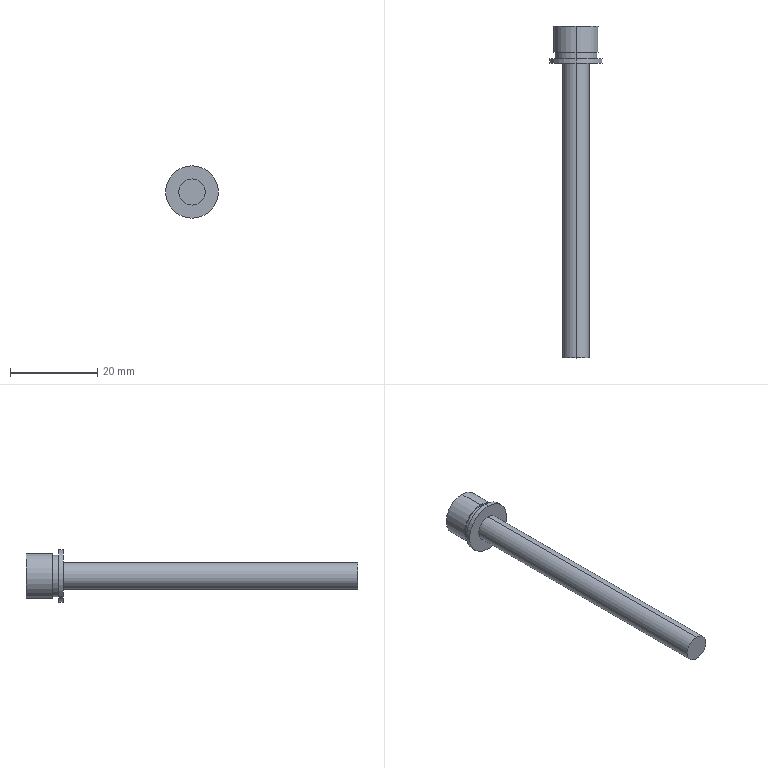Part | SolidWorks | features ICE 3, Revolution 1 | 3 solids | 26 faces | box 12 x 76 x 12 mm | volume 2512 mm3 | plane 14 | cylinder 12 | commonest cylinder face diameters 6 x6 9.6 x2 10.2 x2 12 x2
STEP:
#1=CARTESIAN_POINT('',(0.,-70.,3.));
#2=VERTEX_POINT('',#1);
#3=CARTESIAN_POINT('',(0.,-70.,-3.));
#4=VERTEX_POINT('',#3);
#5=CARTESIAN_POINT('',(0.,-70.,0.));
#6=DIRECTION('',(0.,1.,0.));
#7=DIRECTION('',(0.,0.,1.));
#8=AXIS2_PLACEMENT_3D('',#5,#6,#7);
#9=CIRCLE('',#8,3.);
#10=EDGE_CURVE('',#2,#4,#9,.T.);
#11=ORIENTED_EDGE('',*,*,#10,.T.);
#12=CARTESIAN_POINT('',(0.,0.,-3.));
#13=VERTEX_POINT('',#12);
#14=CARTESIAN_POINT('',(0.,11.322,-3.));
#15=DIRECTION('',(0.,1.,0.));
#16=VECTOR('',#15,1000.);
#17=LINE('',#14,#16);
#18=EDGE_CURVE('',#4,#13,#17,.T.);
#19=ORIENTED_EDGE('',*,*,#18,.T.);
#20=CARTESIAN_POINT('',(0.,0.,3.));
#21=VERTEX_POINT('',#20);
#22=CARTESIAN_POINT('',(0.,0.,0.));
#23=DIRECTION('',(0.,1.,0.));
#24=DIRECTION('',(0.,0.,1.));
#25=AXIS2_PLACEMENT_3D('',#22,#23,#24);
#26=CIRCLE('',#25,3.);
#27=EDGE_CURVE('',#21,#13,#26,.T.);
#28=ORIENTED_EDGE('',*,*,#27,.F.);
#29=CARTESIAN_POINT('',(0.,11.322,3.));
#30=DIRECTION('',(0.,1.,0.));
#31=VECTOR('',#30,1000.);
#32=LINE('',#29,#31);
#33=EDGE_CURVE('',#2,#21,#32,.T.);
#34=ORIENTED_EDGE('',*,*,#33,.F.);
#35=EDGE_LOOP('',(#11,#19,#28,#34));
#36=FACE_OUTER_BOUND('',#35,.T.);
#37=CARTESIAN_POINT('',(0.,11.322,0.));
#38=DIRECTION('',(0.,1.,0.));
#39=DIRECTION('',(0.,0.,1.));
#40=AXIS2_PLACEMENT_3D('',#37,#38,#39);
#41=CYLINDRICAL_SURFACE('',#40,3.);
#42=ADVANCED_FACE('',(#36),#41,.T.);
#43=CARTESIAN_POINT('',(0.,0.,5.1));
#44=VERTEX_POINT('',#43);
#45=CARTESIAN_POINT('',(0.,0.,-5.1));
#46=VERTEX_POINT('',#45);
#47=CARTESIAN_POINT('',(0.,0.,0.));
#48=DIRECTION('',(0.,1.,0.));
#49=DIRECTION('',(0.,0.,1.));
#50=AXIS2_PLACEMENT_3D('',#47,#48,#49);
#51=CIRCLE('',#50,5.1);
#52=EDGE_CURVE('',#44,#46,#51,.T.);
#53=ORIENTED_EDGE('',*,*,#52,.T.);
#54=CARTESIAN_POINT('',(0.,6.,-5.1));
#55=VERTEX_POINT('',#54);
#56=CARTESIAN_POINT('',(0.,11.322,-5.1));
#57=DIRECTION('',(0.,1.,0.));
#58=VECTOR('',#57,1000.);
#59=LINE('',#56,#58);
#60=EDGE_CURVE('',#46,#55,#59,.T.);
#61=ORIENTED_EDGE('',*,*,#60,.T.);
#62=CARTESIAN_POINT('',(0.,6.,5.1));
#63=VERTEX_POINT('',#62);
#64=CARTESIAN_POINT('',(0.,6.,0.));
#65=DIRECTION('',(0.,1.,0.));
#66=DIRECTION('',(0.,0.,1.));
#67=AXIS2_PLACEMENT_3D('',#64,#65,#66);
#68=CIRCLE('',#67,5.1);
#69=EDGE_CURVE('',#63,#55,#68,.T.);
#70=ORIENTED_EDGE('',*,*,#69,.F.);
#71=CARTESIAN_POINT('',(0.,11.322,5.1));
#72=DIRECTION('',(0.,1.,0.));
#73=VECTOR('',#72,1000.);
#74=LINE('',#71,#73);
#75=EDGE_CURVE('',#44,#63,#74,.T.);
#76=ORIENTED_EDGE('',*,*,#75,.F.);
#77=EDGE_LOOP('',(#53,#61,#70,#76));
#78=FACE_OUTER_BOUND('',#77,.T.);
#79=CARTESIAN_POINT('',(0.,11.322,0.));
#80=DIRECTION('',(0.,1.,0.));
#81=DIRECTION('',(0.,0.,1.));
#82=AXIS2_PLACEMENT_3D('',#79,#80,#81);
#83=CYLINDRICAL_SURFACE('',#82,5.1);
#84=ADVANCED_FACE('',(#78),#83,.T.);
#85=CARTESIAN_POINT('',(2.5,6.,-1.443));
#86=VERTEX_POINT('',#85);
#87=CARTESIAN_POINT('',(0.,6.,-2.887));
#88=VERTEX_POINT('',#87);
#89=CARTESIAN_POINT('',(2.5,6.,-1.443));
#90=DIRECTION('',(-0.866,0.,-0.5));
#91=VECTOR('',#90,1000.);
#92=LINE('',#89,#91);
#93=EDGE_CURVE('',#86,#88,#92,.T.);
#94=ORIENTED_EDGE('',*,*,#93,.F.);
#95=CARTESIAN_POINT('',(2.5,6.,1.443));
#96=VERTEX_POINT('',#95);
#97=CARTESIAN_POINT('',(2.5,6.,1.443));
#98=DIRECTION('',(0.,0.,-1.));
#99=VECTOR('',#98,1000.);
#100=LINE('',#97,#99);
#101=EDGE_CURVE('',#96,#86,#100,.T.);
#102=ORIENTED_EDGE('',*,*,#101,.F.);
#103=CARTESIAN_POINT('',(0.,6.,2.887));
#104=VERTEX_POINT('',#103);
#105=CARTESIAN_POINT('',(0.,6.,2.887));
#106=DIRECTION('',(0.866,0.,-0.5));
#107=VECTOR('',#106,1000.);
#108=LINE('',#105,#107);
#109=EDGE_CURVE('',#104,#96,#108,.T.);
#110=ORIENTED_EDGE('',*,*,#109,.F.);
#111=CARTESIAN_POINT('',(-2.5,6.,1.443));
#112=VERTEX_POINT('',#111);
#113=CARTESIAN_POINT('',(-2.5,6.,1.443));
#114=DIRECTION('',(0.866,0.,0.5));
#115=VECTOR('',#114,1000.);
#116=LINE('',#113,#115);
#117=EDGE_CURVE('',#112,#104,#116,.T.);
#118=ORIENTED_EDGE('',*,*,#117,.F.);
#119=CARTESIAN_POINT('',(-2.5,6.,-1.443));
#120=VERTEX_POINT('',#119);
#121=CARTESIAN_POINT('',(-2.5,6.,-1.443));
#122=DIRECTION('',(0.,0.,1.));
#123=VECTOR('',#122,1000.);
#124=LINE('',#121,#123);
#125=EDGE_CURVE('',#120,#112,#124,.T.);
#126=ORIENTED_EDGE('',*,*,#125,.F.);
#127=CARTESIAN_POINT('',(0.,6.,-2.887));
#128=DIRECTION('',(-0.866,0.,0.5));
#129=VECTOR('',#128,1000.);
#130=LINE('',#127,#129);
#131=EDGE_CURVE('',#88,#120,#130,.T.);
#132=ORIENTED_EDGE('',*,*,#131,.F.);
#133=EDGE_LOOP('',(#94,#102,#110,#118,#126,#132));
#134=FACE_BOUND('',#133,.T.);
#135=ORIENTED_EDGE('',*,*,#69,.T.);
#136=CARTESIAN_POINT('',(0.,6.,0.));
#137=DIRECTION('',(0.,1.,0.));
#138=DIRECTION('',(0.,0.,1.));
#139=AXIS2_PLACEMENT_3D('',#136,#137,#138);
#140=CIRCLE('',#139,5.1);
#141=EDGE_CURVE('',#55,#63,#140,.T.);
#142=ORIENTED_EDGE('',*,*,#141,.T.);
#143=EDGE_LOOP('',(#135,#142));
#144=FACE_OUTER_BOUND('',#143,.T.);
#145=CARTESIAN_POINT('',(0.,6.,0.));
#146=DIRECTION('',(0.,1.,0.));
#147=DIRECTION('',(0.,0.,1.));
#148=AXIS2_PLACEMENT_3D('',#145,#146,#147);
#149=PLANE('',#148);
#150=ADVANCED_FACE('',(#134,#144),#149,.T.);
#151=ORIENTED_EDGE('',*,*,#60,.F.);
#152=CARTESIAN_POINT('',(0.,0.,0.));
#153=DIRECTION('',(0.,1.,0.));
#154=DIRECTION('',(0.,0.,1.));
#155=AXIS2_PLACEMENT_3D('',#152,#153,#154);
#156=CIRCLE('',#155,5.1);
#157=EDGE_CURVE('',#46,#44,#156,.T.);
#158=ORIENTED_EDGE('',*,*,#157,.T.);
#159=ORIENTED_EDGE('',*,*,#75,.T.);
#160=ORIENTED_EDGE('',*,*,#141,.F.);
#161=EDGE_LOOP('',(#151,#158,#159,#160));
#162=FACE_OUTER_BOUND('',#161,.T.);
#163=CARTESIAN_POINT('',(0.,11.322,0.));
#164=DIRECTION('',(0.,1.,0.));
#165=DIRECTION('',(0.,0.,1.));
#166=AXIS2_PLACEMENT_3D('',#163,#164,#165);
#167=CYLINDRICAL_SURFACE('',#166,5.1);
#168=ADVANCED_FACE('',(#162),#167,.T.);
#169=ORIENTED_EDGE('',*,*,#27,.T.);
#170=CARTESIAN_POINT('',(0.,0.,0.));
#171=DIRECTION('',(0.,1.,0.));
#172=DIRECTION('',(0.,0.,1.));
#173=AXIS2_PLACEMENT_3D('',#170,#171,#172);
#174=CIRCLE('',#173,3.);
#175=EDGE_CURVE('',#13,#21,#174,.T.);
#176=ORIENTED_EDGE('',*,*,#175,.T.);
#177=EDGE_LOOP('',(#169,#176));
#178=FACE_BOUND('',#177,.T.);
#179=ORIENTED_EDGE('',*,*,#52,.F.);
#180=ORIENTED_EDGE('',*,*,#157,.F.);
#181=EDGE_LOOP('',(#179,#180));
#182=FACE_OUTER_BOUND('',#181,.T.);
#183=CARTESIAN_POINT('',(-5.1,0.,0.));
#184=DIRECTION('',(0.,-1.,0.));
#185=DIRECTION('',(0.,0.,-1.));
#186=AXIS2_PLACEMENT_3D('',#183,#184,#185);
#187=PLANE('',#186);
#188=ADVANCED_FACE('',(#178,#182),#187,.T.);
#189=ORIENTED_EDGE('',*,*,#18,.F.);
#190=CARTESIAN_POINT('',(0.,-70.,0.));
#191=DIRECTION('',(0.,1.,0.));
#192=DIRECTION('',(0.,0.,1.));
#193=AXIS2_PLACEMENT_3D('',#190,#191,#192);
#194=CIRCLE('',#193,3.);
#195=EDGE_CURVE('',#4,#2,#194,.T.);
#196=ORIENTED_EDGE('',*,*,#195,.T.);
#197=ORIENTED_EDGE('',*,*,#33,.T.);
#198=ORIENTED_EDGE('',*,*,#175,.F.);
#199=EDGE_LOOP('',(#189,#196,#197,#198));
#200=FACE_OUTER_BOUND('',#199,.T.);
#201=CARTESIAN_POINT('',(0.,11.322,0.));
#202=DIRECTION('',(0.,1.,0.));
#203=DIRECTION('',(0.,0.,1.));
#204=AXIS2_PLACEMENT_3D('',#201,#202,#203);
#205=CYLINDRICAL_SURFACE('',#204,3.);
#206=ADVANCED_FACE('',(#200),#205,.T.);
#207=ORIENTED_EDGE('',*,*,#10,.F.);
#208=ORIENTED_EDGE('',*,*,#195,.F.);
#209=EDGE_LOOP('',(#207,#208));
#210=FACE_OUTER_BOUND('',#209,.T.);
#211=CARTESIAN_POINT('',(-3.,-70.,0.));
#212=DIRECTION('',(0.,-1.,0.));
#213=DIRECTION('',(0.,0.,-1.));
#214=AXIS2_PLACEMENT_3D('',#211,#212,#213);
#215=PLANE('',#214);
#216=ADVANCED_FACE('',(#210),#215,.T.);
#217=ORIENTED_EDGE('',*,*,#93,.T.);
#218=CARTESIAN_POINT('',(0.,1.,-2.887));
#219=VERTEX_POINT('',#218);
#220=CARTESIAN_POINT('',(0.,1.,-2.887));
#221=DIRECTION('',(0.,1.,0.));
#222=VECTOR('',#221,1000.);
#223=LINE('',#220,#222);
#224=EDGE_CURVE('',#219,#88,#223,.T.);
#225=ORIENTED_EDGE('',*,*,#224,.F.);
#226=CARTESIAN_POINT('',(2.5,1.,-1.443));
#227=VERTEX_POINT('',#226);
#228=CARTESIAN_POINT('',(2.5,1.,-1.443));
#229=DIRECTION('',(-0.866,0.,-0.5));
#230=VECTOR('',#229,1000.);
#231=LINE('',#228,#230);
#232=EDGE_CURVE('',#227,#219,#231,.T.);
#233=ORIENTED_EDGE('',*,*,#232,.F.);
#234=CARTESIAN_POINT('',(2.5,1.,-1.443));
#235=DIRECTION('',(0.,1.,0.));
#236=VECTOR('',#235,1000.);
#237=LINE('',#234,#236);
#238=EDGE_CURVE('',#227,#86,#237,.T.);
#239=ORIENTED_EDGE('',*,*,#238,.T.);
#240=EDGE_LOOP('',(#217,#225,#233,#239));
#241=FACE_OUTER_BOUND('',#240,.T.);
#242=CARTESIAN_POINT('',(2.5,1.,-1.443));
#243=DIRECTION('',(0.5,0.,-0.866));
#244=DIRECTION('',(-0.866,0.,-0.5));
#245=AXIS2_PLACEMENT_3D('',#242,#243,#244);
#246=PLANE('',#245);
#247=ADVANCED_FACE('',(#241),#246,.F.);
#248=ORIENTED_EDGE('',*,*,#101,.T.);
#249=ORIENTED_EDGE('',*,*,#238,.F.);
#250=CARTESIAN_POINT('',(2.5,1.,1.443));
#251=VERTEX_POINT('',#250);
#252=CARTESIAN_POINT('',(2.5,1.,1.443));
#253=DIRECTION('',(0.,0.,-1.));
#254=VECTOR('',#253,1000.);
#255=LINE('',#252,#254);
#256=EDGE_CURVE('',#251,#227,#255,.T.);
#257=ORIENTED_EDGE('',*,*,#256,.F.);
#258=CARTESIAN_POINT('',(2.5,1.,1.443));
#259=DIRECTION('',(0.,1.,0.));
#260=VECTOR('',#259,1000.);
#261=LINE('',#258,#260);
#262=EDGE_CURVE('',#251,#96,#261,.T.);
#263=ORIENTED_EDGE('',*,*,#262,.T.);
#264=EDGE_LOOP('',(#248,#249,#257,#263));
#265=FACE_OUTER_BOUND('',#264,.T.);
#266=CARTESIAN_POINT('',(2.5,1.,1.443));
#267=DIRECTION('',(1.,0.,0.));
#268=DIRECTION('',(0.,0.,-1.));
#269=AXIS2_PLACEMENT_3D('',#266,#267,#268);
#270=PLANE('',#269);
#271=ADVANCED_FACE('',(#265),#270,.F.);
#272=ORIENTED_EDGE('',*,*,#109,.T.);
#273=ORIENTED_EDGE('',*,*,#262,.F.);
#274=CARTESIAN_POINT('',(0.,1.,2.887));
#275=VERTEX_POINT('',#274);
#276=CARTESIAN_POINT('',(0.,1.,2.887));
#277=DIRECTION('',(0.866,0.,-0.5));
#278=VECTOR('',#277,1000.);
#279=LINE('',#276,#278);
#280=EDGE_CURVE('',#275,#251,#279,.T.);
#281=ORIENTED_EDGE('',*,*,#280,.F.);
#282=CARTESIAN_POINT('',(0.,1.,2.887));
#283=DIRECTION('',(0.,1.,0.));
#284=VECTOR('',#283,1000.);
#285=LINE('',#282,#284);
#286=EDGE_CURVE('',#275,#104,#285,.T.);
#287=ORIENTED_EDGE('',*,*,#286,.T.);
#288=EDGE_LOOP('',(#272,#273,#281,#287));
#289=FACE_OUTER_BOUND('',#288,.T.);
#290=CARTESIAN_POINT('',(0.,1.,2.887));
#291=DIRECTION('',(0.5,0.,0.866));
#292=DIRECTION('',(0.866,0.,-0.5));
#293=AXIS2_PLACEMENT_3D('',#290,#291,#292);
#294=PLANE('',#293);
#295=ADVANCED_FACE('',(#289),#294,.F.);
#296=ORIENTED_EDGE('',*,*,#117,.T.);
#297=ORIENTED_EDGE('',*,*,#286,.F.);
#298=CARTESIAN_POINT('',(-2.5,1.,1.443));
#299=VERTEX_POINT('',#298);
#300=CARTESIAN_POINT('',(-2.5,1.,1.443));
#301=DIRECTION('',(0.866,0.,0.5));
#302=VECTOR('',#301,1000.);
#303=LINE('',#300,#302);
#304=EDGE_CURVE('',#299,#275,#303,.T.);
#305=ORIENTED_EDGE('',*,*,#304,.F.);
#306=CARTESIAN_POINT('',(-2.5,1.,1.443));
#307=DIRECTION('',(0.,1.,0.));
#308=VECTOR('',#307,1000.);
#309=LINE('',#306,#308);
#310=EDGE_CURVE('',#299,#112,#309,.T.);
#311=ORIENTED_EDGE('',*,*,#310,.T.);
#312=EDGE_LOOP('',(#296,#297,#305,#311));
#313=FACE_OUTER_BOUND('',#312,.T.);
#314=CARTESIAN_POINT('',(-2.5,1.,1.443));
#315=DIRECTION('',(-0.5,0.,0.866));
#316=DIRECTION('',(0.866,0.,0.5));
#317=AXIS2_PLACEMENT_3D('',#314,#315,#316);
#318=PLANE('',#317);
#319=ADVANCED_FACE('',(#313),#318,.F.);
#320=ORIENTED_EDGE('',*,*,#125,.T.);
#321=ORIENTED_EDGE('',*,*,#310,.F.);
#322=CARTESIAN_POINT('',(-2.5,1.,-1.443));
#323=VERTEX_POINT('',#322);
#324=CARTESIAN_POINT('',(-2.5,1.,-1.443));
#325=DIRECTION('',(0.,0.,1.));
#326=VECTOR('',#325,1000.);
#327=LINE('',#324,#326);
#328=EDGE_CURVE('',#323,#299,#327,.T.);
#329=ORIENTED_EDGE('',*,*,#328,.F.);
#330=CARTESIAN_POINT('',(-2.5,1.,-1.443));
#331=DIRECTION('',(0.,1.,0.));
#332=VECTOR('',#331,1000.);
#333=LINE('',#330,#332);
#334=EDGE_CURVE('',#323,#120,#333,.T.);
#335=ORIENTED_EDGE('',*,*,#334,.T.);
#336=EDGE_LOOP('',(#320,#321,#329,#335));
#337=FACE_OUTER_BOUND('',#336,.T.);
#338=CARTESIAN_POINT('',(-2.5,1.,-1.443));
#339=DIRECTION('',(-1.,0.,0.));
#340=DIRECTION('',(0.,0.,1.));
#341=AXIS2_PLACEMENT_3D('',#338,#339,#340);
#342=PLANE('',#341);
#343=ADVANCED_FACE('',(#337),#342,.F.);
#344=ORIENTED_EDGE('',*,*,#131,.T.);
#345=ORIENTED_EDGE('',*,*,#334,.F.);
#346=CARTESIAN_POINT('',(0.,1.,-2.887));
#347=DIRECTION('',(-0.866,0.,0.5));
#348=VECTOR('',#347,1000.);
#349=LINE('',#346,#348);
#350=EDGE_CURVE('',#219,#323,#349,.T.);
#351=ORIENTED_EDGE('',*,*,#350,.F.);
#352=ORIENTED_EDGE('',*,*,#224,.T.);
#353=EDGE_LOOP('',(#344,#345,#351,#352));
#354=FACE_OUTER_BOUND('',#353,.T.);
#355=CARTESIAN_POINT('',(0.,1.,-2.887));
#356=DIRECTION('',(-0.5,0.,-0.866));
#357=DIRECTION('',(-0.866,0.,0.5));
#358=AXIS2_PLACEMENT_3D('',#355,#356,#357);
#359=PLANE('',#358);
#360=ADVANCED_FACE('',(#354),#359,.F.);
#361=ORIENTED_EDGE('',*,*,#232,.T.);
#362=ORIENTED_EDGE('',*,*,#350,.T.);
#363=ORIENTED_EDGE('',*,*,#328,.T.);
#364=ORIENTED_EDGE('',*,*,#304,.T.);
#365=ORIENTED_EDGE('',*,*,#280,.T.);
#366=ORIENTED_EDGE('',*,*,#256,.T.);
#367=EDGE_LOOP('',(#361,#362,#363,#364,#365,#366));
#368=FACE_OUTER_BOUND('',#367,.T.);
#369=CARTESIAN_POINT('',(0.,1.,0.));
#370=DIRECTION('',(0.,1.,0.));
#371=DIRECTION('',(0.,0.,1.));
#372=AXIS2_PLACEMENT_3D('',#369,#370,#371);
#373=PLANE('',#372);
#374=ADVANCED_FACE('',(#368),#373,.T.);
#375=CLOSED_SHELL('',(#42,#84,#150,#168,#188,#206,#216,#247,#271,#295,#319,#343,#360,#374));
#376=MANIFOLD_SOLID_BREP('',#375);
#377=CARTESIAN_POINT('',(0.,-1.5,3.));
#378=VERTEX_POINT('',#377);
#379=CARTESIAN_POINT('',(0.,-1.5,-3.));
#380=VERTEX_POINT('',#379);
#381=CARTESIAN_POINT('',(0.,-1.5,0.));
#382=DIRECTION('',(0.,-1.,0.));
#383=DIRECTION('',(0.,0.,-1.));
#384=AXIS2_PLACEMENT_3D('',#381,#382,#383);
#385=CIRCLE('',#384,3.);
#386=EDGE_CURVE('',#378,#380,#385,.T.);
#387=ORIENTED_EDGE('',*,*,#386,.T.);
#388=CARTESIAN_POINT('',(0.,0.,-3.));
#389=VERTEX_POINT('',#388);
#390=CARTESIAN_POINT('',(0.,-1.5,-3.));
#391=DIRECTION('',(0.,1.,0.));
#392=VECTOR('',#391,1000.);
#393=LINE('',#390,#392);
#394=EDGE_CURVE('',#380,#389,#393,.T.);
#395=ORIENTED_EDGE('',*,*,#394,.T.);
#396=CARTESIAN_POINT('',(0.,0.,3.));
#397=VERTEX_POINT('',#396);
#398=CARTESIAN_POINT('',(0.,0.,0.));
#399=DIRECTION('',(0.,-1.,0.));
#400=DIRECTION('',(0.,0.,-1.));
#401=AXIS2_PLACEMENT_3D('',#398,#399,#400);
#402=CIRCLE('',#401,3.);
#403=EDGE_CURVE('',#397,#389,#402,.T.);
#404=ORIENTED_EDGE('',*,*,#403,.F.);
#405=CARTESIAN_POINT('',(0.,-1.5,3.));
#406=DIRECTION('',(0.,1.,0.));
#407=VECTOR('',#406,1000.);
#408=LINE('',#405,#407);
#409=EDGE_CURVE('',#378,#397,#408,.T.);
#410=ORIENTED_EDGE('',*,*,#409,.F.);
#411=EDGE_LOOP('',(#387,#395,#404,#410));
#412=FACE_OUTER_BOUND('',#411,.T.);
#413=CARTESIAN_POINT('',(0.,-1.5,0.));
#414=DIRECTION('',(0.,1.,0.));
#415=DIRECTION('',(0.,0.,1.));
#416=AXIS2_PLACEMENT_3D('',#413,#414,#415);
#417=CYLINDRICAL_SURFACE('',#416,3.);
#418=ADVANCED_FACE('',(#412),#417,.F.);
#419=CARTESIAN_POINT('',(0.,-1.5,-4.8));
#420=VERTEX_POINT('',#419);
#421=CARTESIAN_POINT('',(0.,-1.5,4.8));
#422=VERTEX_POINT('',#421);
#423=CARTESIAN_POINT('',(0.,-1.5,0.));
#424=DIRECTION('',(0.,-1.,0.));
#425=DIRECTION('',(0.,0.,-1.));
#426=AXIS2_PLACEMENT_3D('',#423,#424,#425);
#427=CIRCLE('',#426,4.8);
#428=EDGE_CURVE('',#420,#422,#427,.T.);
#429=ORIENTED_EDGE('',*,*,#428,.F.);
#430=CARTESIAN_POINT('',(0.,0.,-4.8));
#431=VERTEX_POINT('',#430);
#432=CARTESIAN_POINT('',(0.,-1.5,-4.8));
#433=DIRECTION('',(0.,1.,0.));
#434=VECTOR('',#433,1000.);
#435=LINE('',#432,#434);
#436=EDGE_CURVE('',#420,#431,#435,.T.);
#437=ORIENTED_EDGE('',*,*,#436,.T.);
#438=CARTESIAN_POINT('',(0.,0.,4.8));
#439=VERTEX_POINT('',#438);
#440=CARTESIAN_POINT('',(0.,0.,0.));
#441=DIRECTION('',(0.,-1.,0.));
#442=DIRECTION('',(0.,0.,-1.));
#443=AXIS2_PLACEMENT_3D('',#440,#441,#442);
#444=CIRCLE('',#443,4.8);
#445=EDGE_CURVE('',#431,#439,#444,.T.);
#446=ORIENTED_EDGE('',*,*,#445,.T.);
#447=CARTESIAN_POINT('',(0.,-1.5,4.8));
#448=DIRECTION('',(0.,1.,0.));
#449=VECTOR('',#448,1000.);
#450=LINE('',#447,#449);
#451=EDGE_CURVE('',#422,#439,#450,.T.);
#452=ORIENTED_EDGE('',*,*,#451,.F.);
#453=EDGE_LOOP('',(#429,#437,#446,#452));
#454=FACE_OUTER_BOUND('',#453,.T.);
#455=CARTESIAN_POINT('',(0.,-1.5,0.));
#456=DIRECTION('',(0.,1.,0.));
#457=DIRECTION('',(0.,0.,1.));
#458=AXIS2_PLACEMENT_3D('',#455,#456,#457);
#459=CYLINDRICAL_SURFACE('',#458,4.8);
#460=ADVANCED_FACE('',(#454),#459,.T.);
#461=CARTESIAN_POINT('',(0.,-1.5,0.));
#462=DIRECTION('',(0.,-1.,0.));
#463=DIRECTION('',(0.,0.,-1.));
#464=AXIS2_PLACEMENT_3D('',#461,#462,#463);
#465=CIRCLE('',#464,4.8);
#466=EDGE_CURVE('',#422,#420,#465,.T.);
#467=ORIENTED_EDGE('',*,*,#466,.T.);
#468=ORIENTED_EDGE('',*,*,#428,.T.);
#469=EDGE_LOOP('',(#467,#468));
#470=FACE_OUTER_BOUND('',#469,.T.);
#471=ORIENTED_EDGE('',*,*,#386,.F.);
#472=CARTESIAN_POINT('',(0.,-1.5,0.));
#473=DIRECTION('',(0.,-1.,0.));
#474=DIRECTION('',(0.,0.,-1.));
#475=AXIS2_PLACEMENT_3D('',#472,#473,#474);
#476=CIRCLE('',#475,3.);
#477=EDGE_CURVE('',#380,#378,#476,.T.);
#478=ORIENTED_EDGE('',*,*,#477,.F.);
#479=EDGE_LOOP('',(#471,#478));
#480=FACE_BOUND('',#479,.T.);
#481=CARTESIAN_POINT('',(0.,-1.5,0.));
#482=DIRECTION('',(0.,-1.,0.));
#483=DIRECTION('',(0.,0.,-1.));
#484=AXIS2_PLACEMENT_3D('',#481,#482,#483);
#485=PLANE('',#484);
#486=ADVANCED_FACE('',(#470,#480),#485,.T.);
#487=CARTESIAN_POINT('',(0.,0.,0.));
#488=DIRECTION('',(0.,-1.,0.));
#489=DIRECTION('',(0.,0.,-1.));
#490=AXIS2_PLACEMENT_3D('',#487,#488,#489);
#491=CIRCLE('',#490,4.8);
#492=EDGE_CURVE('',#439,#431,#491,.T.);
#493=ORIENTED_EDGE('',*,*,#492,.F.);
#494=ORIENTED_EDGE('',*,*,#445,.F.);
#495=EDGE_LOOP('',(#493,#494));
#496=FACE_OUTER_BOUND('',#495,.T.);
#497=ORIENTED_EDGE('',*,*,#403,.T.);
#498=CARTESIAN_POINT('',(0.,0.,0.));
#499=DIRECTION('',(0.,-1.,0.));
#500=DIRECTION('',(0.,0.,-1.));
#501=AXIS2_PLACEMENT_3D('',#498,#499,#500);
#502=CIRCLE('',#501,3.);
#503=EDGE_CURVE('',#389,#397,#502,.T.);
#504=ORIENTED_EDGE('',*,*,#503,.T.);
#505=EDGE_LOOP('',(#497,#504));
#506=FACE_BOUND('',#505,.T.);
#507=CARTESIAN_POINT('',(0.,0.,0.));
#508=DIRECTION('',(0.,-1.,0.));
#509=DIRECTION('',(0.,0.,-1.));
#510=AXIS2_PLACEMENT_3D('',#507,#508,#509);
#511=PLANE('',#510);
#512=ADVANCED_FACE('',(#496,#506),#511,.F.);
#513=ORIENTED_EDGE('',*,*,#436,.F.);
#514=ORIENTED_EDGE('',*,*,#466,.F.);
#515=ORIENTED_EDGE('',*,*,#451,.T.);
#516=ORIENTED_EDGE('',*,*,#492,.T.);
#517=EDGE_LOOP('',(#513,#514,#515,#516));
#518=FACE_OUTER_BOUND('',#517,.T.);
#519=CARTESIAN_POINT('',(0.,-1.5,0.));
#520=DIRECTION('',(0.,1.,0.));
#521=DIRECTION('',(0.,0.,1.));
#522=AXIS2_PLACEMENT_3D('',#519,#520,#521);
#523=CYLINDRICAL_SURFACE('',#522,4.8);
#524=ADVANCED_FACE('',(#518),#523,.T.);
#525=ORIENTED_EDGE('',*,*,#394,.F.);
#526=ORIENTED_EDGE('',*,*,#477,.T.);
#527=ORIENTED_EDGE('',*,*,#409,.T.);
#528=ORIENTED_EDGE('',*,*,#503,.F.);
#529=EDGE_LOOP('',(#525,#526,#527,#528));
#530=FACE_OUTER_BOUND('',#529,.T.);
#531=CARTESIAN_POINT('',(0.,-1.5,0.));
#532=DIRECTION('',(0.,1.,0.));
#533=DIRECTION('',(0.,0.,1.));
#534=AXIS2_PLACEMENT_3D('',#531,#532,#533);
#535=CYLINDRICAL_SURFACE('',#534,3.);
#536=ADVANCED_FACE('',(#530),#535,.F.);
#537=CLOSED_SHELL('',(#418,#460,#486,#512,#524,#536));
#538=MANIFOLD_SOLID_BREP('',#537);
#539=CARTESIAN_POINT('',(0.,-2.5,3.));
#540=VERTEX_POINT('',#539);
#541=CARTESIAN_POINT('',(0.,-2.5,-3.));
#542=VERTEX_POINT('',#541);
#543=CARTESIAN_POINT('',(0.,-2.5,0.));
#544=DIRECTION('',(0.,-1.,0.));
#545=DIRECTION('',(0.,0.,-1.));
#546=AXIS2_PLACEMENT_3D('',#543,#544,#545);
#547=CIRCLE('',#546,3.);
#548=EDGE_CURVE('',#540,#542,#547,.T.);
#549=ORIENTED_EDGE('',*,*,#548,.T.);
#550=CARTESIAN_POINT('',(0.,-1.5,-3.));
#551=VERTEX_POINT('',#550);
#552=CARTESIAN_POINT('',(0.,-2.5,-3.));
#553=DIRECTION('',(0.,1.,0.));
#554=VECTOR('',#553,1000.);
#555=LINE('',#552,#554);
#556=EDGE_CURVE('',#542,#551,#555,.T.);
#557=ORIENTED_EDGE('',*,*,#556,.T.);
#558=CARTESIAN_POINT('',(0.,-1.5,3.));
#559=VERTEX_POINT('',#558);
#560=CARTESIAN_POINT('',(0.,-1.5,0.));
#561=DIRECTION('',(0.,-1.,0.));
#562=DIRECTION('',(0.,0.,-1.));
#563=AXIS2_PLACEMENT_3D('',#560,#561,#562);
#564=CIRCLE('',#563,3.);
#565=EDGE_CURVE('',#559,#551,#564,.T.);
#566=ORIENTED_EDGE('',*,*,#565,.F.);
#567=CARTESIAN_POINT('',(0.,-2.5,3.));
#568=DIRECTION('',(0.,1.,0.));
#569=VECTOR('',#568,1000.);
#570=LINE('',#567,#569);
#571=EDGE_CURVE('',#540,#559,#570,.T.);
#572=ORIENTED_EDGE('',*,*,#571,.F.);
#573=EDGE_LOOP('',(#549,#557,#566,#572));
#574=FACE_OUTER_BOUND('',#573,.T.);
#575=CARTESIAN_POINT('',(0.,-2.5,0.));
#576=DIRECTION('',(0.,1.,0.));
#577=DIRECTION('',(0.,0.,1.));
#578=AXIS2_PLACEMENT_3D('',#575,#576,#577);
#579=CYLINDRICAL_SURFACE('',#578,3.);
#580=ADVANCED_FACE('',(#574),#579,.F.);
#581=CARTESIAN_POINT('',(0.,-2.5,-6.));
#582=VERTEX_POINT('',#581);
#583=CARTESIAN_POINT('',(0.,-2.5,6.));
#584=VERTEX_POINT('',#583);
#585=CARTESIAN_POINT('',(0.,-2.5,0.));
#586=DIRECTION('',(0.,-1.,0.));
#587=DIRECTION('',(0.,0.,-1.));
#588=AXIS2_PLACEMENT_3D('',#585,#586,#587);
#589=CIRCLE('',#588,6.);
#590=EDGE_CURVE('',#582,#584,#589,.T.);
#591=ORIENTED_EDGE('',*,*,#590,.F.);
#592=CARTESIAN_POINT('',(0.,-1.5,-6.));
#593=VERTEX_POINT('',#592);
#594=CARTESIAN_POINT('',(0.,-2.5,-6.));
#595=DIRECTION('',(0.,1.,0.));
#596=VECTOR('',#595,1000.);
#597=LINE('',#594,#596);
#598=EDGE_CURVE('',#582,#593,#597,.T.);
#599=ORIENTED_EDGE('',*,*,#598,.T.);
#600=CARTESIAN_POINT('',(0.,-1.5,6.));
#601=VERTEX_POINT('',#600);
#602=CARTESIAN_POINT('',(0.,-1.5,0.));
#603=DIRECTION('',(0.,-1.,0.));
#604=DIRECTION('',(0.,0.,-1.));
#605=AXIS2_PLACEMENT_3D('',#602,#603,#604);
#606=CIRCLE('',#605,6.);
#607=EDGE_CURVE('',#593,#601,#606,.T.);
#608=ORIENTED_EDGE('',*,*,#607,.T.);
#609=CARTESIAN_POINT('',(0.,-2.5,6.));
#610=DIRECTION('',(0.,1.,0.));
#611=VECTOR('',#610,1000.);
#612=LINE('',#609,#611);
#613=EDGE_CURVE('',#584,#601,#612,.T.);
#614=ORIENTED_EDGE('',*,*,#613,.F.);
#615=EDGE_LOOP('',(#591,#599,#608,#614));
#616=FACE_OUTER_BOUND('',#615,.T.);
#617=CARTESIAN_POINT('',(0.,-2.5,0.));
#618=DIRECTION('',(0.,1.,0.));
#619=DIRECTION('',(0.,0.,1.));
#620=AXIS2_PLACEMENT_3D('',#617,#618,#619);
#621=CYLINDRICAL_SURFACE('',#620,6.);
#622=ADVANCED_FACE('',(#616),#621,.T.);
#623=CARTESIAN_POINT('',(0.,-2.5,0.));
#624=DIRECTION('',(0.,-1.,0.));
#625=DIRECTION('',(0.,0.,-1.));
#626=AXIS2_PLACEMENT_3D('',#623,#624,#625);
#627=CIRCLE('',#626,6.);
#628=EDGE_CURVE('',#584,#582,#627,.T.);
#629=ORIENTED_EDGE('',*,*,#628,.T.);
#630=ORIENTED_EDGE('',*,*,#590,.T.);
#631=EDGE_LOOP('',(#629,#630));
#632=FACE_OUTER_BOUND('',#631,.T.);
#633=ORIENTED_EDGE('',*,*,#548,.F.);
#634=CARTESIAN_POINT('',(0.,-2.5,0.));
#635=DIRECTION('',(0.,-1.,0.));
#636=DIRECTION('',(0.,0.,-1.));
#637=AXIS2_PLACEMENT_3D('',#634,#635,#636);
#638=CIRCLE('',#637,3.);
#639=EDGE_CURVE('',#542,#540,#638,.T.);
#640=ORIENTED_EDGE('',*,*,#639,.F.);
#641=EDGE_LOOP('',(#633,#640));
#642=FACE_BOUND('',#641,.T.);
#643=CARTESIAN_POINT('',(0.,-2.5,0.));
#644=DIRECTION('',(0.,-1.,0.));
#645=DIRECTION('',(0.,0.,-1.));
#646=AXIS2_PLACEMENT_3D('',#643,#644,#645);
#647=PLANE('',#646);
#648=ADVANCED_FACE('',(#632,#642),#647,.T.);
#649=CARTESIAN_POINT('',(0.,-1.5,0.));
#650=DIRECTION('',(0.,-1.,0.));
#651=DIRECTION('',(0.,0.,-1.));
#652=AXIS2_PLACEMENT_3D('',#649,#650,#651);
#653=CIRCLE('',#652,6.);
#654=EDGE_CURVE('',#601,#593,#653,.T.);
#655=ORIENTED_EDGE('',*,*,#654,.F.);
#656=ORIENTED_EDGE('',*,*,#607,.F.);
#657=EDGE_LOOP('',(#655,#656));
#658=FACE_OUTER_BOUND('',#657,.T.);
#659=ORIENTED_EDGE('',*,*,#565,.T.);
#660=CARTESIAN_POINT('',(0.,-1.5,0.));
#661=DIRECTION('',(0.,-1.,0.));
#662=DIRECTION('',(0.,0.,-1.));
#663=AXIS2_PLACEMENT_3D('',#660,#661,#662);
#664=CIRCLE('',#663,3.);
#665=EDGE_CURVE('',#551,#559,#664,.T.);
#666=ORIENTED_EDGE('',*,*,#665,.T.);
#667=EDGE_LOOP('',(#659,#666));
#668=FACE_BOUND('',#667,.T.);
#669=CARTESIAN_POINT('',(0.,-1.5,0.));
#670=DIRECTION('',(0.,-1.,0.));
#671=DIRECTION('',(0.,0.,-1.));
#672=AXIS2_PLACEMENT_3D('',#669,#670,#671);
#673=PLANE('',#672);
#674=ADVANCED_FACE('',(#658,#668),#673,.F.);
#675=ORIENTED_EDGE('',*,*,#598,.F.);
#676=ORIENTED_EDGE('',*,*,#628,.F.);
#677=ORIENTED_EDGE('',*,*,#613,.T.);
#678=ORIENTED_EDGE('',*,*,#654,.T.);
#679=EDGE_LOOP('',(#675,#676,#677,#678));
#680=FACE_OUTER_BOUND('',#679,.T.);
#681=CARTESIAN_POINT('',(0.,-2.5,0.));
#682=DIRECTION('',(0.,1.,0.));
#683=DIRECTION('',(0.,0.,1.));
#684=AXIS2_PLACEMENT_3D('',#681,#682,#683);
#685=CYLINDRICAL_SURFACE('',#684,6.);
#686=ADVANCED_FACE('',(#680),#685,.T.);
#687=ORIENTED_EDGE('',*,*,#556,.F.);
#688=ORIENTED_EDGE('',*,*,#639,.T.);
#689=ORIENTED_EDGE('',*,*,#571,.T.);
#690=ORIENTED_EDGE('',*,*,#665,.F.);
#691=EDGE_LOOP('',(#687,#688,#689,#690));
#692=FACE_OUTER_BOUND('',#691,.T.);
#693=CARTESIAN_POINT('',(0.,-2.5,0.));
#694=DIRECTION('',(0.,1.,0.));
#695=DIRECTION('',(0.,0.,1.));
#696=AXIS2_PLACEMENT_3D('',#693,#694,#695);
#697=CYLINDRICAL_SURFACE('',#696,3.);
#698=ADVANCED_FACE('',(#692),#697,.F.);
#699=CLOSED_SHELL('',(#580,#622,#648,#674,#686,#698));
#700=MANIFOLD_SOLID_BREP('',#699);
#701=CARTESIAN_POINT('',(0.,0.,0.));
#702=DIRECTION('',(0.,0.,1.));
#703=DIRECTION('',(1.,0.,0.));
#704=AXIS2_PLACEMENT_3D('',#701,#702,#703);
#705=(LENGTH_UNIT()NAMED_UNIT(*)SI_UNIT(.MILLI.,.METRE.));
#706=UNCERTAINTY_MEASURE_WITH_UNIT(LENGTH_MEASURE(0.00001),#705,'','');
#707=(NAMED_UNIT(*)PLANE_ANGLE_UNIT()SI_UNIT($,.RADIAN.));
#708=(NAMED_UNIT(*)SI_UNIT($,.STERADIAN.)SOLID_ANGLE_UNIT());
#709=(GEOMETRIC_REPRESENTATION_CONTEXT(3)GLOBAL_UNCERTAINTY_ASSIGNED_CONTEXT((#706))GLOBAL_UNIT_ASSIGNED_CONTEXT((#705,#707,#708))REPRESENTATION_CONTEXT('',''));
#710=ADVANCED_BREP_SHAPE_REPRESENTATION('',(#376,#538,#700,#704),#709);